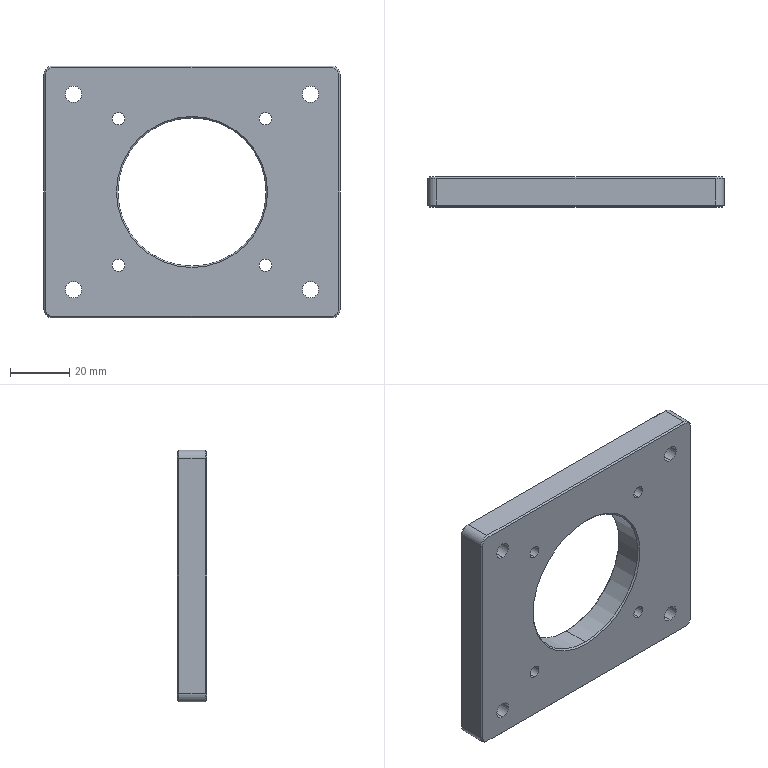Part | STEP file | ND25021-01-JDKM-16-TL | 1 solid | 48 faces | box 100 x 10 x 85 mm | volume 63653 mm3 | cylinder 22 | plane 14 | cone 12 | commonest cylinder face diameters 4.2 x8 5.5 x8 6 x4 50 x2